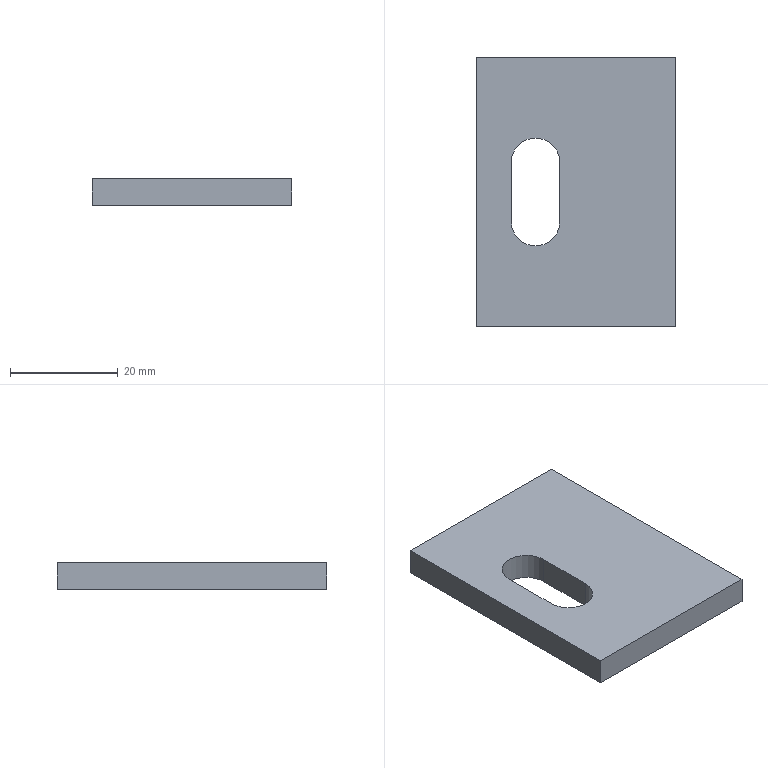Part | SolidWorks | features BaseBody 1 | 1 solid | 10 faces | box 37 x 50 x 5 mm | volume 8437 mm3 | plane 8 | cylinder 2 | commonest cylinder face diameters 9 x2
STEP:
#1=CARTESIAN_POINT('',(-12.,5.5,-5.));
#2=VERTEX_POINT('',#1);
#3=CARTESIAN_POINT('',(-12.,5.5,0.));
#4=VERTEX_POINT('',#3);
#5=CARTESIAN_POINT('',(-12.,5.5,-10.));
#6=DIRECTION('',(0.,0.,1.));
#7=VECTOR('',#6,1000.);
#8=LINE('',#5,#7);
#9=EDGE_CURVE('',#2,#4,#8,.T.);
#10=ORIENTED_EDGE('',*,*,#9,.T.);
#11=CARTESIAN_POINT('',(-12.,-5.5,0.));
#12=VERTEX_POINT('',#11);
#13=CARTESIAN_POINT('',(-12.,5.5,0.));
#14=DIRECTION('',(0.,-1.,0.));
#15=VECTOR('',#14,1000.);
#16=LINE('',#13,#15);
#17=EDGE_CURVE('',#4,#12,#16,.T.);
#18=ORIENTED_EDGE('',*,*,#17,.T.);
#19=CARTESIAN_POINT('',(-12.,-5.5,-5.));
#20=VERTEX_POINT('',#19);
#21=CARTESIAN_POINT('',(-12.,-5.5,-10.));
#22=DIRECTION('',(0.,0.,1.));
#23=VECTOR('',#22,1000.);
#24=LINE('',#21,#23);
#25=EDGE_CURVE('',#20,#12,#24,.T.);
#26=ORIENTED_EDGE('',*,*,#25,.F.);
#27=CARTESIAN_POINT('',(-12.,0.,-5.));
#28=DIRECTION('',(0.,-1.,0.));
#29=VECTOR('',#28,1000.);
#30=LINE('',#27,#29);
#31=EDGE_CURVE('',#2,#20,#30,.T.);
#32=ORIENTED_EDGE('',*,*,#31,.F.);
#33=EDGE_LOOP('',(#10,#18,#26,#32));
#34=FACE_OUTER_BOUND('',#33,.T.);
#35=CARTESIAN_POINT('',(-12.,5.5,-10.));
#36=DIRECTION('',(-1.,0.,0.));
#37=DIRECTION('',(0.,1.,0.));
#38=AXIS2_PLACEMENT_3D('',#35,#36,#37);
#39=PLANE('',#38);
#40=ADVANCED_FACE('',(#34),#39,.F.);
#41=ORIENTED_EDGE('',*,*,#25,.T.);
#42=CARTESIAN_POINT('',(-3.,-5.5,0.));
#43=VERTEX_POINT('',#42);
#44=CARTESIAN_POINT('',(-7.5,-5.5,0.));
#45=DIRECTION('',(0.,0.,1.));
#46=DIRECTION('',(1.,0.,0.));
#47=AXIS2_PLACEMENT_3D('',#44,#45,#46);
#48=CIRCLE('',#47,4.5);
#49=EDGE_CURVE('',#12,#43,#48,.T.);
#50=ORIENTED_EDGE('',*,*,#49,.T.);
#51=CARTESIAN_POINT('',(-3.,-5.5,-5.));
#52=VERTEX_POINT('',#51);
#53=CARTESIAN_POINT('',(-3.,-5.5,-10.));
#54=DIRECTION('',(0.,0.,1.));
#55=VECTOR('',#54,1000.);
#56=LINE('',#53,#55);
#57=EDGE_CURVE('',#52,#43,#56,.T.);
#58=ORIENTED_EDGE('',*,*,#57,.F.);
#59=CARTESIAN_POINT('',(-7.5,-5.5,-5.));
#60=DIRECTION('',(0.,0.,1.));
#61=DIRECTION('',(1.,0.,0.));
#62=AXIS2_PLACEMENT_3D('',#59,#60,#61);
#63=CIRCLE('',#62,4.5);
#64=EDGE_CURVE('',#20,#52,#63,.T.);
#65=ORIENTED_EDGE('',*,*,#64,.F.);
#66=EDGE_LOOP('',(#41,#50,#58,#65));
#67=FACE_OUTER_BOUND('',#66,.T.);
#68=CARTESIAN_POINT('',(-7.5,-5.5,-10.));
#69=DIRECTION('',(0.,0.,1.));
#70=DIRECTION('',(1.,0.,0.));
#71=AXIS2_PLACEMENT_3D('',#68,#69,#70);
#72=CYLINDRICAL_SURFACE('',#71,4.5);
#73=ADVANCED_FACE('',(#67),#72,.F.);
#74=ORIENTED_EDGE('',*,*,#57,.T.);
#75=CARTESIAN_POINT('',(-3.,5.5,0.));
#76=VERTEX_POINT('',#75);
#77=CARTESIAN_POINT('',(-3.,5.5,0.));
#78=DIRECTION('',(0.,1.,0.));
#79=VECTOR('',#78,1000.);
#80=LINE('',#77,#79);
#81=EDGE_CURVE('',#43,#76,#80,.T.);
#82=ORIENTED_EDGE('',*,*,#81,.T.);
#83=CARTESIAN_POINT('',(-3.,5.5,-5.));
#84=VERTEX_POINT('',#83);
#85=CARTESIAN_POINT('',(-3.,5.5,-10.));
#86=DIRECTION('',(0.,0.,1.));
#87=VECTOR('',#86,1000.);
#88=LINE('',#85,#87);
#89=EDGE_CURVE('',#84,#76,#88,.T.);
#90=ORIENTED_EDGE('',*,*,#89,.F.);
#91=CARTESIAN_POINT('',(-3.,0.,-5.));
#92=DIRECTION('',(0.,1.,0.));
#93=VECTOR('',#92,1000.);
#94=LINE('',#91,#93);
#95=EDGE_CURVE('',#52,#84,#94,.T.);
#96=ORIENTED_EDGE('',*,*,#95,.F.);
#97=EDGE_LOOP('',(#74,#82,#90,#96));
#98=FACE_OUTER_BOUND('',#97,.T.);
#99=CARTESIAN_POINT('',(-3.,5.5,-10.));
#100=DIRECTION('',(1.,0.,0.));
#101=DIRECTION('',(0.,1.,0.));
#102=AXIS2_PLACEMENT_3D('',#99,#100,#101);
#103=PLANE('',#102);
#104=ADVANCED_FACE('',(#98),#103,.F.);
#105=ORIENTED_EDGE('',*,*,#89,.T.);
#106=CARTESIAN_POINT('',(-7.5,5.5,0.));
#107=DIRECTION('',(0.,0.,1.));
#108=DIRECTION('',(1.,0.,0.));
#109=AXIS2_PLACEMENT_3D('',#106,#107,#108);
#110=CIRCLE('',#109,4.5);
#111=EDGE_CURVE('',#76,#4,#110,.T.);
#112=ORIENTED_EDGE('',*,*,#111,.T.);
#113=ORIENTED_EDGE('',*,*,#9,.F.);
#114=CARTESIAN_POINT('',(-7.5,5.5,-5.));
#115=DIRECTION('',(0.,0.,1.));
#116=DIRECTION('',(1.,0.,0.));
#117=AXIS2_PLACEMENT_3D('',#114,#115,#116);
#118=CIRCLE('',#117,4.5);
#119=EDGE_CURVE('',#84,#2,#118,.T.);
#120=ORIENTED_EDGE('',*,*,#119,.F.);
#121=EDGE_LOOP('',(#105,#112,#113,#120));
#122=FACE_OUTER_BOUND('',#121,.T.);
#123=CARTESIAN_POINT('',(-7.5,5.5,-10.));
#124=DIRECTION('',(0.,0.,1.));
#125=DIRECTION('',(1.,0.,0.));
#126=AXIS2_PLACEMENT_3D('',#123,#124,#125);
#127=CYLINDRICAL_SURFACE('',#126,4.5);
#128=ADVANCED_FACE('',(#122),#127,.F.);
#129=ORIENTED_EDGE('',*,*,#111,.F.);
#130=ORIENTED_EDGE('',*,*,#81,.F.);
#131=ORIENTED_EDGE('',*,*,#49,.F.);
#132=ORIENTED_EDGE('',*,*,#17,.F.);
#133=EDGE_LOOP('',(#129,#130,#131,#132));
#134=FACE_BOUND('',#133,.T.);
#135=CARTESIAN_POINT('',(18.5,-25.,0.));
#136=VERTEX_POINT('',#135);
#137=CARTESIAN_POINT('',(18.5,25.,0.));
#138=VERTEX_POINT('',#137);
#139=CARTESIAN_POINT('',(18.5,25.,0.));
#140=DIRECTION('',(0.,1.,0.));
#141=VECTOR('',#140,1000.);
#142=LINE('',#139,#141);
#143=EDGE_CURVE('',#136,#138,#142,.T.);
#144=ORIENTED_EDGE('',*,*,#143,.T.);
#145=CARTESIAN_POINT('',(-18.5,25.,0.));
#146=VERTEX_POINT('',#145);
#147=CARTESIAN_POINT('',(-18.5,25.,0.));
#148=DIRECTION('',(-1.,0.,0.));
#149=VECTOR('',#148,1000.);
#150=LINE('',#147,#149);
#151=EDGE_CURVE('',#138,#146,#150,.T.);
#152=ORIENTED_EDGE('',*,*,#151,.T.);
#153=CARTESIAN_POINT('',(-18.5,-25.,0.));
#154=VERTEX_POINT('',#153);
#155=CARTESIAN_POINT('',(-18.5,25.,0.));
#156=DIRECTION('',(0.,-1.,0.));
#157=VECTOR('',#156,1000.);
#158=LINE('',#155,#157);
#159=EDGE_CURVE('',#146,#154,#158,.T.);
#160=ORIENTED_EDGE('',*,*,#159,.T.);
#161=CARTESIAN_POINT('',(-18.5,-25.,0.));
#162=DIRECTION('',(1.,0.,0.));
#163=VECTOR('',#162,1000.);
#164=LINE('',#161,#163);
#165=EDGE_CURVE('',#154,#136,#164,.T.);
#166=ORIENTED_EDGE('',*,*,#165,.T.);
#167=EDGE_LOOP('',(#144,#152,#160,#166));
#168=FACE_OUTER_BOUND('',#167,.T.);
#169=CARTESIAN_POINT('',(0.,0.,0.));
#170=DIRECTION('',(0.,0.,1.));
#171=DIRECTION('',(1.,0.,0.));
#172=AXIS2_PLACEMENT_3D('',#169,#170,#171);
#173=PLANE('',#172);
#174=ADVANCED_FACE('',(#134,#168),#173,.T.);
#175=ORIENTED_EDGE('',*,*,#95,.T.);
#176=ORIENTED_EDGE('',*,*,#119,.T.);
#177=ORIENTED_EDGE('',*,*,#31,.T.);
#178=ORIENTED_EDGE('',*,*,#64,.T.);
#179=EDGE_LOOP('',(#175,#176,#177,#178));
#180=FACE_BOUND('',#179,.T.);
#181=CARTESIAN_POINT('',(18.5,-25.,-5.));
#182=VERTEX_POINT('',#181);
#183=CARTESIAN_POINT('',(18.5,25.,-5.));
#184=VERTEX_POINT('',#183);
#185=CARTESIAN_POINT('',(18.5,25.,-5.));
#186=DIRECTION('',(0.,1.,0.));
#187=VECTOR('',#186,1000.);
#188=LINE('',#185,#187);
#189=EDGE_CURVE('',#182,#184,#188,.T.);
#190=ORIENTED_EDGE('',*,*,#189,.F.);
#191=CARTESIAN_POINT('',(-18.5,-25.,-5.));
#192=VERTEX_POINT('',#191);
#193=CARTESIAN_POINT('',(-18.5,-25.,-5.));
#194=DIRECTION('',(1.,0.,0.));
#195=VECTOR('',#194,1000.);
#196=LINE('',#193,#195);
#197=EDGE_CURVE('',#192,#182,#196,.T.);
#198=ORIENTED_EDGE('',*,*,#197,.F.);
#199=CARTESIAN_POINT('',(-18.5,25.,-5.));
#200=VERTEX_POINT('',#199);
#201=CARTESIAN_POINT('',(-18.5,25.,-5.));
#202=DIRECTION('',(0.,-1.,0.));
#203=VECTOR('',#202,1000.);
#204=LINE('',#201,#203);
#205=EDGE_CURVE('',#200,#192,#204,.T.);
#206=ORIENTED_EDGE('',*,*,#205,.F.);
#207=CARTESIAN_POINT('',(-18.5,25.,-5.));
#208=DIRECTION('',(-1.,0.,0.));
#209=VECTOR('',#208,1000.);
#210=LINE('',#207,#209);
#211=EDGE_CURVE('',#184,#200,#210,.T.);
#212=ORIENTED_EDGE('',*,*,#211,.F.);
#213=EDGE_LOOP('',(#190,#198,#206,#212));
#214=FACE_OUTER_BOUND('',#213,.T.);
#215=CARTESIAN_POINT('',(0.,0.,-5.));
#216=DIRECTION('',(0.,0.,1.));
#217=DIRECTION('',(1.,0.,0.));
#218=AXIS2_PLACEMENT_3D('',#215,#216,#217);
#219=PLANE('',#218);
#220=ADVANCED_FACE('',(#180,#214),#219,.F.);
#221=ORIENTED_EDGE('',*,*,#151,.F.);
#222=CARTESIAN_POINT('',(18.5,25.,-5.));
#223=DIRECTION('',(0.,0.,1.));
#224=VECTOR('',#223,1000.);
#225=LINE('',#222,#224);
#226=EDGE_CURVE('',#184,#138,#225,.T.);
#227=ORIENTED_EDGE('',*,*,#226,.F.);
#228=ORIENTED_EDGE('',*,*,#211,.T.);
#229=CARTESIAN_POINT('',(-18.5,25.,-5.));
#230=DIRECTION('',(0.,0.,1.));
#231=VECTOR('',#230,1000.);
#232=LINE('',#229,#231);
#233=EDGE_CURVE('',#200,#146,#232,.T.);
#234=ORIENTED_EDGE('',*,*,#233,.T.);
#235=EDGE_LOOP('',(#221,#227,#228,#234));
#236=FACE_OUTER_BOUND('',#235,.T.);
#237=CARTESIAN_POINT('',(-18.5,25.,-5.));
#238=DIRECTION('',(0.,1.,0.));
#239=DIRECTION('',(1.,0.,0.));
#240=AXIS2_PLACEMENT_3D('',#237,#238,#239);
#241=PLANE('',#240);
#242=ADVANCED_FACE('',(#236),#241,.T.);
#243=ORIENTED_EDGE('',*,*,#159,.F.);
#244=ORIENTED_EDGE('',*,*,#233,.F.);
#245=ORIENTED_EDGE('',*,*,#205,.T.);
#246=CARTESIAN_POINT('',(-18.5,-25.,-5.));
#247=DIRECTION('',(0.,0.,1.));
#248=VECTOR('',#247,1000.);
#249=LINE('',#246,#248);
#250=EDGE_CURVE('',#192,#154,#249,.T.);
#251=ORIENTED_EDGE('',*,*,#250,.T.);
#252=EDGE_LOOP('',(#243,#244,#245,#251));
#253=FACE_OUTER_BOUND('',#252,.T.);
#254=CARTESIAN_POINT('',(-18.5,25.,-5.));
#255=DIRECTION('',(-1.,0.,0.));
#256=DIRECTION('',(0.,1.,0.));
#257=AXIS2_PLACEMENT_3D('',#254,#255,#256);
#258=PLANE('',#257);
#259=ADVANCED_FACE('',(#253),#258,.T.);
#260=ORIENTED_EDGE('',*,*,#165,.F.);
#261=ORIENTED_EDGE('',*,*,#250,.F.);
#262=ORIENTED_EDGE('',*,*,#197,.T.);
#263=CARTESIAN_POINT('',(18.5,-25.,-5.));
#264=DIRECTION('',(0.,0.,1.));
#265=VECTOR('',#264,1000.);
#266=LINE('',#263,#265);
#267=EDGE_CURVE('',#182,#136,#266,.T.);
#268=ORIENTED_EDGE('',*,*,#267,.T.);
#269=EDGE_LOOP('',(#260,#261,#262,#268));
#270=FACE_OUTER_BOUND('',#269,.T.);
#271=CARTESIAN_POINT('',(-18.5,-25.,-5.));
#272=DIRECTION('',(0.,-1.,0.));
#273=DIRECTION('',(0.,0.,-1.));
#274=AXIS2_PLACEMENT_3D('',#271,#272,#273);
#275=PLANE('',#274);
#276=ADVANCED_FACE('',(#270),#275,.T.);
#277=ORIENTED_EDGE('',*,*,#143,.F.);
#278=ORIENTED_EDGE('',*,*,#267,.F.);
#279=ORIENTED_EDGE('',*,*,#189,.T.);
#280=ORIENTED_EDGE('',*,*,#226,.T.);
#281=EDGE_LOOP('',(#277,#278,#279,#280));
#282=FACE_OUTER_BOUND('',#281,.T.);
#283=CARTESIAN_POINT('',(18.5,25.,-5.));
#284=DIRECTION('',(1.,0.,0.));
#285=DIRECTION('',(0.,1.,0.));
#286=AXIS2_PLACEMENT_3D('',#283,#284,#285);
#287=PLANE('',#286);
#288=ADVANCED_FACE('',(#282),#287,.T.);
#289=CLOSED_SHELL('',(#40,#73,#104,#128,#174,#220,#242,#259,#276,#288));
#290=MANIFOLD_SOLID_BREP('',#289);
#291=CARTESIAN_POINT('',(0.,0.,0.));
#292=DIRECTION('',(0.,0.,1.));
#293=DIRECTION('',(1.,0.,0.));
#294=AXIS2_PLACEMENT_3D('',#291,#292,#293);
#295=(LENGTH_UNIT()NAMED_UNIT(*)SI_UNIT(.MILLI.,.METRE.));
#296=UNCERTAINTY_MEASURE_WITH_UNIT(LENGTH_MEASURE(0.00001),#295,'','');
#297=(NAMED_UNIT(*)PLANE_ANGLE_UNIT()SI_UNIT($,.RADIAN.));
#298=(NAMED_UNIT(*)SI_UNIT($,.STERADIAN.)SOLID_ANGLE_UNIT());
#299=(GEOMETRIC_REPRESENTATION_CONTEXT(3)GLOBAL_UNCERTAINTY_ASSIGNED_CONTEXT((#296))GLOBAL_UNIT_ASSIGNED_CONTEXT((#295,#297,#298))REPRESENTATION_CONTEXT('',''));
#300=ADVANCED_BREP_SHAPE_REPRESENTATION('',(#290,#294),#299);